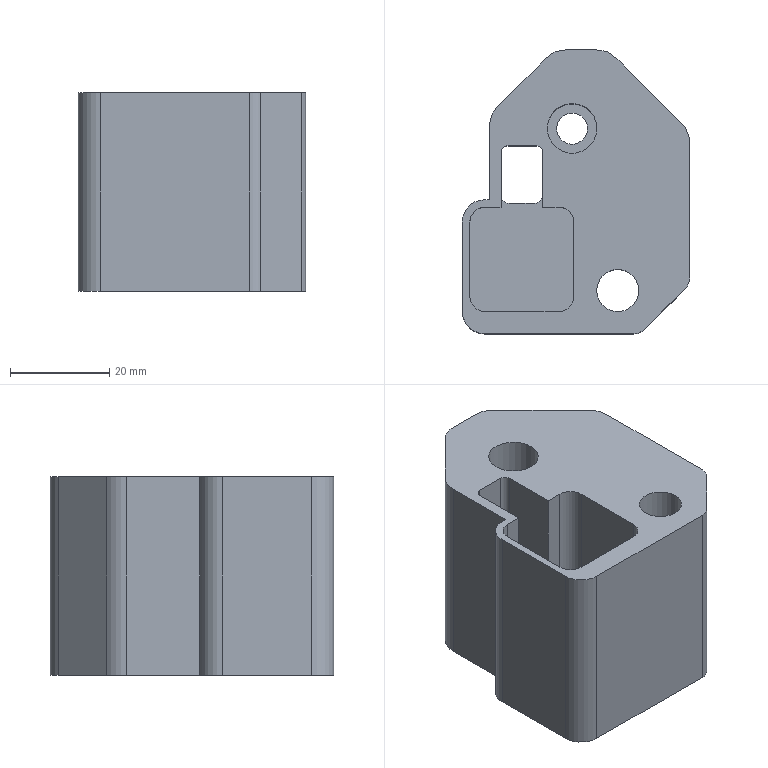Part | NX | features PS-6 2 | 1 solid | 49 faces | box 45.815 x 57.187 x 40 mm | volume 60835 mm3 | plane 27 | cylinder 22 | commonest cylinder face diameters 6 x6 11 x4 2.4 x2 3.4 x2 8 x2 9 x2